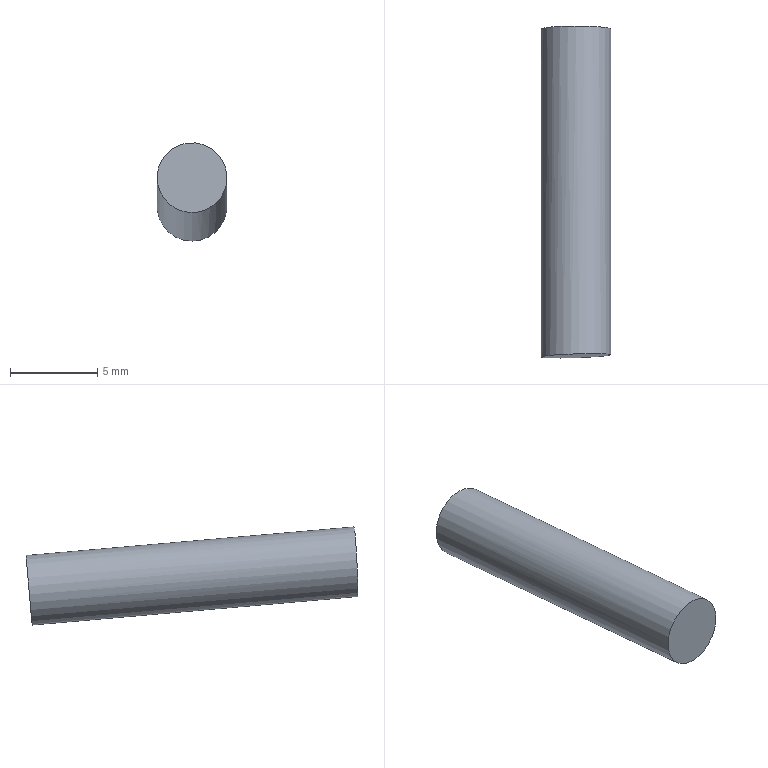Part | NX | features solid 2 | 1 solid | 3 faces | box 4 x 19.02 x 5.629 mm | volume 236.161 mm3 | plane 2 | cylinder 1 | commonest cylinder face diameters 4 x1
STEP:
#1=CARTESIAN_POINT('',(-227.901,-39.47,-43.613));
#2=VERTEX_POINT('',#1);
#3=CARTESIAN_POINT('',(-227.901,-39.295,-41.621));
#4=DIRECTION('',(0.,-0.9962,0.08716));
#5=DIRECTION('',(0.,-0.08716,-0.9962));
#6=AXIS2_PLACEMENT_3D('',#3,#4,#5);
#7=CIRCLE('',#6,2.);
#8=EDGE_CURVE('',#2,#2,#7,.T.);
#9=ORIENTED_EDGE('',*,*,#8,.F.);
#10=EDGE_LOOP('',(#9));
#11=FACE_BOUND('',#10,.T.);
#12=CARTESIAN_POINT('',(-228.366,-38.62,-33.907));
#13=DIRECTION('',(0.,-0.9962,0.08716));
#14=DIRECTION('',(0.,-0.08716,-0.9962));
#15=AXIS2_PLACEMENT_3D('',#12,#13,#14);
#16=PLANE('',#15);
#17=ADVANCED_FACE('',(#11),#16,.F.);
#18=CARTESIAN_POINT('',(-226.521,-58.049,-41.433));
#19=VERTEX_POINT('',#18);
#20=CARTESIAN_POINT('',(-227.901,-58.017,-39.983));
#21=DIRECTION('',(-0.03252,0.9981,-0.05307));
#22=DIRECTION('',(0.6892,-0.01607,-0.7244));
#23=AXIS2_PLACEMENT_3D('',#20,#21,#22);
#24=ELLIPSE('',#23,2.002,2.);
#25=EDGE_CURVE('',#19,#19,#24,.T.);
#26=ORIENTED_EDGE('',*,*,#25,.F.);
#27=EDGE_LOOP('',(#26));
#28=FACE_BOUND('',#27,.T.);
#29=CARTESIAN_POINT('',(-422.194,-57.948,80.353));
#30=DIRECTION('',(-0.03252,0.9981,-0.05307));
#31=DIRECTION('',(0.05223,-0.05133,-0.9973));
#32=AXIS2_PLACEMENT_3D('',#29,#30,#31);
#33=PLANE('',#32);
#34=ADVANCED_FACE('',(#28),#33,.F.);
#35=ORIENTED_EDGE('',*,*,#8,.T.);
#36=EDGE_LOOP('',(#35));
#37=FACE_BOUND('',#36,.T.);
#38=ORIENTED_EDGE('',*,*,#25,.T.);
#39=EDGE_LOOP('',(#38));
#40=FACE_BOUND('',#39,.T.);
#41=CARTESIAN_POINT('',(-227.901,-58.702,-39.923));
#42=DIRECTION('',(0.,0.9962,-0.08716));
#43=DIRECTION('',(-0.9997,-0.001977,-0.0226));
#44=AXIS2_PLACEMENT_3D('',#41,#42,#43);
#45=CYLINDRICAL_SURFACE('',#44,2.);
#46=ADVANCED_FACE('',(#37,#40),#45,.T.);
#47=CLOSED_SHELL('',(#17,#34,#46));
#48=MANIFOLD_SOLID_BREP('',#47);
#49=(LENGTH_UNIT()NAMED_UNIT(*)SI_UNIT(.MILLI.,.METRE.));
#50=UNCERTAINTY_MEASURE_WITH_UNIT(LENGTH_MEASURE(0.00001),#49,'','');
#51=(NAMED_UNIT(*)PLANE_ANGLE_UNIT()SI_UNIT($,.RADIAN.));
#52=(NAMED_UNIT(*)SI_UNIT($,.STERADIAN.)SOLID_ANGLE_UNIT());
#53=(GEOMETRIC_REPRESENTATION_CONTEXT(3)GLOBAL_UNCERTAINTY_ASSIGNED_CONTEXT((#50))GLOBAL_UNIT_ASSIGNED_CONTEXT((#49,#51,#52))REPRESENTATION_CONTEXT('',''));
#54=ADVANCED_BREP_SHAPE_REPRESENTATION('',(#48),#53);